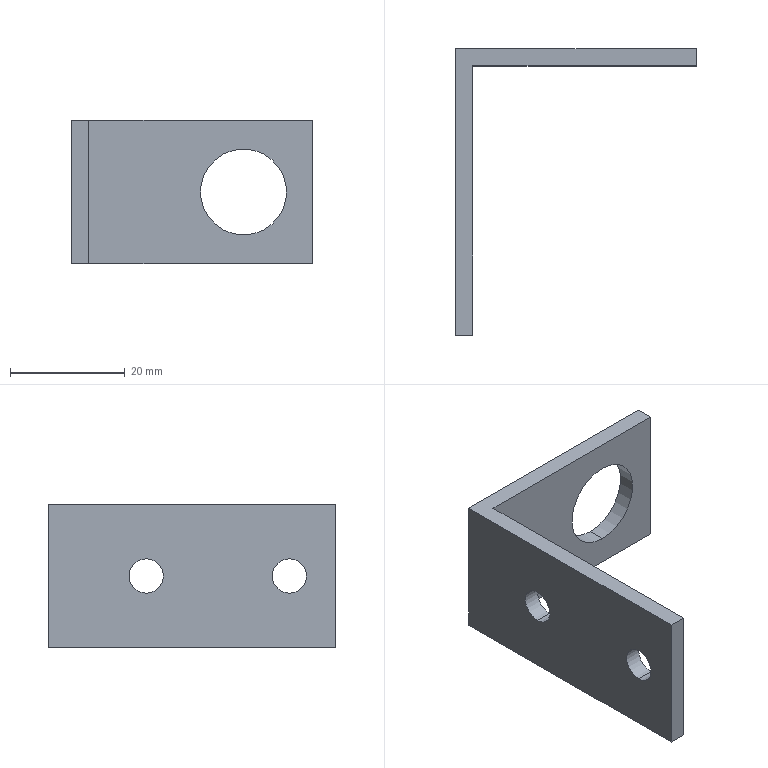Part | STEP file | 1 solid | 14 faces | box 42 x 50 x 25 mm | volume 5975 mm3 | plane 8 | cylinder 6 | commonest cylinder face diameters 6 x4 15 x2
STEP:
#1=CARTESIAN_POINT('',(0.,0.,0.));
#2=DIRECTION('',(0.,0.,1.));
#3=DIRECTION('',(1.,0.,0.));
#4=AXIS2_PLACEMENT_3D('',#1,#2,#3);
#5=CARTESIAN_POINT('',(0.,-17.,-3.));
#6=VERTEX_POINT('',#5);
#7=CARTESIAN_POINT('',(3.,-17.,-3.));
#8=VERTEX_POINT('',#7);
#9=CARTESIAN_POINT('',(25.,-17.,-3.));
#10=DIRECTION('',(1.,0.,0.));
#11=VECTOR('',#10,1.);
#12=LINE('',#9,#11);
#13=CARTESIAN_POINT('',(25.,-17.,0.));
#14=DIRECTION('',(1.,0.,0.));
#15=DIRECTION('',(0.,0.,-1.));
#16=AXIS2_PLACEMENT_3D('',#13,#14,#15);
#17=CYLINDRICAL_SURFACE('',#16,3.);
#18=CARTESIAN_POINT('',(6.283,0.));
#19=DIRECTION('',(0.,1.));
#20=VECTOR('',#19,1.);
#21=LINE('',#18,#20);
#22=(GEOMETRIC_REPRESENTATION_CONTEXT(2)PARAMETRIC_REPRESENTATION_CONTEXT()REPRESENTATION_CONTEXT('',''));
#23=DEFINITIONAL_REPRESENTATION('',(#21),#22);
#24=PCURVE('',#17,#23);
#25=CARTESIAN_POINT('',(25.,-17.,0.));
#26=DIRECTION('',(1.,0.,0.));
#27=DIRECTION('',(0.,0.,-1.));
#28=AXIS2_PLACEMENT_3D('',#25,#26,#27);
#29=CYLINDRICAL_SURFACE('',#28,3.);
#30=CARTESIAN_POINT('',(0.,0.));
#31=DIRECTION('',(0.,1.));
#32=VECTOR('',#31,1.);
#33=LINE('',#30,#32);
#34=(GEOMETRIC_REPRESENTATION_CONTEXT(2)PARAMETRIC_REPRESENTATION_CONTEXT()REPRESENTATION_CONTEXT('',''));
#35=DEFINITIONAL_REPRESENTATION('',(#33),#34);
#36=PCURVE('',#29,#35);
#37=SURFACE_CURVE('',#12,(#24,#36),.PCURVE_S1.);
#38=EDGE_CURVE('',#6,#8,#37,.T.);
#39=ORIENTED_EDGE('',*,*,#38,.T.);
#40=CARTESIAN_POINT('',(3.,-17.,3.));
#41=VERTEX_POINT('',#40);
#42=CARTESIAN_POINT('',(3.,-17.,0.));
#43=DIRECTION('',(-1.,0.,0.));
#44=DIRECTION('',(0.,0.,-1.));
#45=AXIS2_PLACEMENT_3D('',#42,#43,#44);
#46=CIRCLE('',#45,3.);
#47=CARTESIAN_POINT('',(6.283,-22.));
#48=DIRECTION('',(-1.,0.));
#49=VECTOR('',#48,1.);
#50=LINE('',#47,#49);
#51=(GEOMETRIC_REPRESENTATION_CONTEXT(2)PARAMETRIC_REPRESENTATION_CONTEXT()REPRESENTATION_CONTEXT('',''));
#52=DEFINITIONAL_REPRESENTATION('',(#50),#51);
#53=PCURVE('',#17,#52);
#54=CARTESIAN_POINT('',(3.,0.,-12.5));
#55=DIRECTION('',(-1.,0.,0.));
#56=DIRECTION('',(0.,-1.,0.));
#57=AXIS2_PLACEMENT_3D('',#54,#55,#56);
#58=PLANE('',#57);
#59=CARTESIAN_POINT('',(17.,12.5));
#60=DIRECTION('',(0.,-1.));
#61=AXIS2_PLACEMENT_2D('',#59,#60);
#62=CIRCLE('',#61,3.);
#63=(GEOMETRIC_REPRESENTATION_CONTEXT(2)PARAMETRIC_REPRESENTATION_CONTEXT()REPRESENTATION_CONTEXT('',''));
#64=DEFINITIONAL_REPRESENTATION('',(#62),#63);
#65=PCURVE('',#58,#64);
#66=SURFACE_CURVE('',#46,(#53,#65),.PCURVE_S1.);
#67=EDGE_CURVE('',#8,#41,#66,.T.);
#68=ORIENTED_EDGE('',*,*,#67,.T.);
#69=CARTESIAN_POINT('',(0.,-17.,3.));
#70=VERTEX_POINT('',#69);
#71=CARTESIAN_POINT('',(25.,-17.,3.));
#72=DIRECTION('',(1.,0.,0.));
#73=VECTOR('',#72,1.);
#74=LINE('',#71,#73);
#75=CARTESIAN_POINT('',(3.142,0.));
#76=DIRECTION('',(0.,1.));
#77=VECTOR('',#76,1.);
#78=LINE('',#75,#77);
#79=(GEOMETRIC_REPRESENTATION_CONTEXT(2)PARAMETRIC_REPRESENTATION_CONTEXT()REPRESENTATION_CONTEXT('',''));
#80=DEFINITIONAL_REPRESENTATION('',(#78),#79);
#81=PCURVE('',#17,#80);
#82=CARTESIAN_POINT('',(3.142,0.));
#83=DIRECTION('',(0.,1.));
#84=VECTOR('',#83,1.);
#85=LINE('',#82,#84);
#86=(GEOMETRIC_REPRESENTATION_CONTEXT(2)PARAMETRIC_REPRESENTATION_CONTEXT()REPRESENTATION_CONTEXT('',''));
#87=DEFINITIONAL_REPRESENTATION('',(#85),#86);
#88=PCURVE('',#29,#87);
#89=SURFACE_CURVE('',#74,(#81,#88),.PCURVE_S1.);
#90=EDGE_CURVE('',#70,#41,#89,.T.);
#91=ORIENTED_EDGE('',*,*,#90,.F.);
#92=CARTESIAN_POINT('',(0.,-17.,0.));
#93=DIRECTION('',(1.,0.,0.));
#94=DIRECTION('',(0.,0.,-1.));
#95=AXIS2_PLACEMENT_3D('',#92,#93,#94);
#96=CIRCLE('',#95,3.);
#97=CARTESIAN_POINT('',(0.,-25.));
#98=DIRECTION('',(1.,0.));
#99=VECTOR('',#98,1.);
#100=LINE('',#97,#99);
#101=(GEOMETRIC_REPRESENTATION_CONTEXT(2)PARAMETRIC_REPRESENTATION_CONTEXT()REPRESENTATION_CONTEXT('',''));
#102=DEFINITIONAL_REPRESENTATION('',(#100),#101);
#103=PCURVE('',#17,#102);
#104=CARTESIAN_POINT('',(0.,0.,-12.5));
#105=DIRECTION('',(-1.,0.,0.));
#106=DIRECTION('',(0.,-1.,0.));
#107=AXIS2_PLACEMENT_3D('',#104,#105,#106);
#108=PLANE('',#107);
#109=CARTESIAN_POINT('',(17.,9.5));
#110=CARTESIAN_POINT('',(11.804,9.5));
#111=CARTESIAN_POINT('',(14.402,14.));
#112=CARTESIAN_POINT('',(17.,18.5));
#113=CARTESIAN_POINT('',(19.598,14.));
#114=CARTESIAN_POINT('',(22.196,9.5));
#115=CARTESIAN_POINT('',(17.,9.5));
#116=(BOUNDED_CURVE()B_SPLINE_CURVE(2,(#109,#110,#111,#112,#113,#114,#115),.UNSPECIFIED.,.T.,.F.)B_SPLINE_CURVE_WITH_KNOTS((1,2,2,2,2,1),(-2.094,0.,2.094,4.189,6.283,8.378),.UNSPECIFIED.)CURVE()GEOMETRIC_REPRESENTATION_ITEM()RATIONAL_B_SPLINE_CURVE((1.,0.5,1.,0.5,1.,0.5,1.))REPRESENTATION_ITEM(''));
#117=(GEOMETRIC_REPRESENTATION_CONTEXT(2)PARAMETRIC_REPRESENTATION_CONTEXT()REPRESENTATION_CONTEXT('',''));
#118=DEFINITIONAL_REPRESENTATION('',(#116),#117);
#119=PCURVE('',#108,#118);
#120=SURFACE_CURVE('',#96,(#103,#119),.PCURVE_S1.);
#121=EDGE_CURVE('',#70,#6,#120,.T.);
#122=ORIENTED_EDGE('',*,*,#121,.T.);
#123=EDGE_LOOP('',(#39,#68,#91,#122));
#124=FACE_BOUND('',#123,.F.);
#125=ADVANCED_FACE('',(#124),#17,.F.);
#126=CARTESIAN_POINT('',(0.,-42.,-3.));
#127=VERTEX_POINT('',#126);
#128=CARTESIAN_POINT('',(3.,-42.,-3.));
#129=VERTEX_POINT('',#128);
#130=CARTESIAN_POINT('',(25.,-42.,-3.));
#131=DIRECTION('',(1.,0.,0.));
#132=VECTOR('',#131,1.);
#133=LINE('',#130,#132);
#134=CARTESIAN_POINT('',(25.,-42.,0.));
#135=DIRECTION('',(1.,0.,0.));
#136=DIRECTION('',(0.,0.,-1.));
#137=AXIS2_PLACEMENT_3D('',#134,#135,#136);
#138=CYLINDRICAL_SURFACE('',#137,3.);
#139=CARTESIAN_POINT('',(6.283,0.));
#140=DIRECTION('',(0.,1.));
#141=VECTOR('',#140,1.);
#142=LINE('',#139,#141);
#143=(GEOMETRIC_REPRESENTATION_CONTEXT(2)PARAMETRIC_REPRESENTATION_CONTEXT()REPRESENTATION_CONTEXT('',''));
#144=DEFINITIONAL_REPRESENTATION('',(#142),#143);
#145=PCURVE('',#138,#144);
#146=CARTESIAN_POINT('',(25.,-42.,0.));
#147=DIRECTION('',(1.,0.,0.));
#148=DIRECTION('',(0.,0.,-1.));
#149=AXIS2_PLACEMENT_3D('',#146,#147,#148);
#150=CYLINDRICAL_SURFACE('',#149,3.);
#151=CARTESIAN_POINT('',(0.,0.));
#152=DIRECTION('',(0.,1.));
#153=VECTOR('',#152,1.);
#154=LINE('',#151,#153);
#155=(GEOMETRIC_REPRESENTATION_CONTEXT(2)PARAMETRIC_REPRESENTATION_CONTEXT()REPRESENTATION_CONTEXT('',''));
#156=DEFINITIONAL_REPRESENTATION('',(#154),#155);
#157=PCURVE('',#150,#156);
#158=SURFACE_CURVE('',#133,(#145,#157),.PCURVE_S1.);
#159=EDGE_CURVE('',#127,#129,#158,.T.);
#160=ORIENTED_EDGE('',*,*,#159,.T.);
#161=CARTESIAN_POINT('',(3.,-42.,3.));
#162=VERTEX_POINT('',#161);
#163=CARTESIAN_POINT('',(3.,-42.,0.));
#164=DIRECTION('',(-1.,0.,0.));
#165=DIRECTION('',(0.,0.,-1.));
#166=AXIS2_PLACEMENT_3D('',#163,#164,#165);
#167=CIRCLE('',#166,3.);
#168=CARTESIAN_POINT('',(6.283,-22.));
#169=DIRECTION('',(-1.,0.));
#170=VECTOR('',#169,1.);
#171=LINE('',#168,#170);
#172=(GEOMETRIC_REPRESENTATION_CONTEXT(2)PARAMETRIC_REPRESENTATION_CONTEXT()REPRESENTATION_CONTEXT('',''));
#173=DEFINITIONAL_REPRESENTATION('',(#171),#172);
#174=PCURVE('',#138,#173);
#175=CARTESIAN_POINT('',(42.,12.5));
#176=DIRECTION('',(0.,-1.));
#177=AXIS2_PLACEMENT_2D('',#175,#176);
#178=CIRCLE('',#177,3.);
#179=(GEOMETRIC_REPRESENTATION_CONTEXT(2)PARAMETRIC_REPRESENTATION_CONTEXT()REPRESENTATION_CONTEXT('',''));
#180=DEFINITIONAL_REPRESENTATION('',(#178),#179);
#181=PCURVE('',#58,#180);
#182=SURFACE_CURVE('',#167,(#174,#181),.PCURVE_S1.);
#183=EDGE_CURVE('',#129,#162,#182,.T.);
#184=ORIENTED_EDGE('',*,*,#183,.T.);
#185=CARTESIAN_POINT('',(0.,-42.,3.));
#186=VERTEX_POINT('',#185);
#187=CARTESIAN_POINT('',(25.,-42.,3.));
#188=DIRECTION('',(1.,0.,0.));
#189=VECTOR('',#188,1.);
#190=LINE('',#187,#189);
#191=CARTESIAN_POINT('',(3.142,0.));
#192=DIRECTION('',(0.,1.));
#193=VECTOR('',#192,1.);
#194=LINE('',#191,#193);
#195=(GEOMETRIC_REPRESENTATION_CONTEXT(2)PARAMETRIC_REPRESENTATION_CONTEXT()REPRESENTATION_CONTEXT('',''));
#196=DEFINITIONAL_REPRESENTATION('',(#194),#195);
#197=PCURVE('',#138,#196);
#198=CARTESIAN_POINT('',(3.142,0.));
#199=DIRECTION('',(0.,1.));
#200=VECTOR('',#199,1.);
#201=LINE('',#198,#200);
#202=(GEOMETRIC_REPRESENTATION_CONTEXT(2)PARAMETRIC_REPRESENTATION_CONTEXT()REPRESENTATION_CONTEXT('',''));
#203=DEFINITIONAL_REPRESENTATION('',(#201),#202);
#204=PCURVE('',#150,#203);
#205=SURFACE_CURVE('',#190,(#197,#204),.PCURVE_S1.);
#206=EDGE_CURVE('',#186,#162,#205,.T.);
#207=ORIENTED_EDGE('',*,*,#206,.F.);
#208=CARTESIAN_POINT('',(0.,-42.,0.));
#209=DIRECTION('',(1.,0.,0.));
#210=DIRECTION('',(0.,0.,-1.));
#211=AXIS2_PLACEMENT_3D('',#208,#209,#210);
#212=CIRCLE('',#211,3.);
#213=CARTESIAN_POINT('',(0.,-25.));
#214=DIRECTION('',(1.,0.));
#215=VECTOR('',#214,1.);
#216=LINE('',#213,#215);
#217=(GEOMETRIC_REPRESENTATION_CONTEXT(2)PARAMETRIC_REPRESENTATION_CONTEXT()REPRESENTATION_CONTEXT('',''));
#218=DEFINITIONAL_REPRESENTATION('',(#216),#217);
#219=PCURVE('',#138,#218);
#220=CARTESIAN_POINT('',(42.,9.5));
#221=CARTESIAN_POINT('',(36.804,9.5));
#222=CARTESIAN_POINT('',(39.402,14.));
#223=CARTESIAN_POINT('',(42.,18.5));
#224=CARTESIAN_POINT('',(44.598,14.));
#225=CARTESIAN_POINT('',(47.196,9.5));
#226=CARTESIAN_POINT('',(42.,9.5));
#227=(BOUNDED_CURVE()B_SPLINE_CURVE(2,(#220,#221,#222,#223,#224,#225,#226),.UNSPECIFIED.,.T.,.F.)B_SPLINE_CURVE_WITH_KNOTS((1,2,2,2,2,1),(-2.094,0.,2.094,4.189,6.283,8.378),.UNSPECIFIED.)CURVE()GEOMETRIC_REPRESENTATION_ITEM()RATIONAL_B_SPLINE_CURVE((1.,0.5,1.,0.5,1.,0.5,1.))REPRESENTATION_ITEM(''));
#228=(GEOMETRIC_REPRESENTATION_CONTEXT(2)PARAMETRIC_REPRESENTATION_CONTEXT()REPRESENTATION_CONTEXT('',''));
#229=DEFINITIONAL_REPRESENTATION('',(#227),#228);
#230=PCURVE('',#108,#229);
#231=SURFACE_CURVE('',#212,(#219,#230),.PCURVE_S1.);
#232=EDGE_CURVE('',#186,#127,#231,.T.);
#233=ORIENTED_EDGE('',*,*,#232,.T.);
#234=EDGE_LOOP('',(#160,#184,#207,#233));
#235=FACE_BOUND('',#234,.F.);
#236=ADVANCED_FACE('',(#235),#138,.F.);
#237=CARTESIAN_POINT('',(30.,0.,-7.5));
#238=VERTEX_POINT('',#237);
#239=CARTESIAN_POINT('',(30.,-3.,-7.5));
#240=VERTEX_POINT('',#239);
#241=CARTESIAN_POINT('',(30.,-25.,-7.5));
#242=DIRECTION('',(0.,-1.,0.));
#243=VECTOR('',#242,1.);
#244=LINE('',#241,#243);
#245=CARTESIAN_POINT('',(30.,-25.,0.));
#246=DIRECTION('',(0.,-1.,0.));
#247=DIRECTION('',(0.,0.,-1.));
#248=AXIS2_PLACEMENT_3D('',#245,#246,#247);
#249=CYLINDRICAL_SURFACE('',#248,7.5);
#250=CARTESIAN_POINT('',(6.283,0.));
#251=DIRECTION('',(0.,1.));
#252=VECTOR('',#251,1.);
#253=LINE('',#250,#252);
#254=(GEOMETRIC_REPRESENTATION_CONTEXT(2)PARAMETRIC_REPRESENTATION_CONTEXT()REPRESENTATION_CONTEXT('',''));
#255=DEFINITIONAL_REPRESENTATION('',(#253),#254);
#256=PCURVE('',#249,#255);
#257=CARTESIAN_POINT('',(30.,-25.,0.));
#258=DIRECTION('',(0.,-1.,0.));
#259=DIRECTION('',(0.,0.,-1.));
#260=AXIS2_PLACEMENT_3D('',#257,#258,#259);
#261=CYLINDRICAL_SURFACE('',#260,7.5);
#262=CARTESIAN_POINT('',(0.,0.));
#263=DIRECTION('',(0.,1.));
#264=VECTOR('',#263,1.);
#265=LINE('',#262,#264);
#266=(GEOMETRIC_REPRESENTATION_CONTEXT(2)PARAMETRIC_REPRESENTATION_CONTEXT()REPRESENTATION_CONTEXT('',''));
#267=DEFINITIONAL_REPRESENTATION('',(#265),#266);
#268=PCURVE('',#261,#267);
#269=SURFACE_CURVE('',#244,(#256,#268),.PCURVE_S1.);
#270=EDGE_CURVE('',#238,#240,#269,.T.);
#271=ORIENTED_EDGE('',*,*,#270,.T.);
#272=CARTESIAN_POINT('',(30.,-3.,7.5));
#273=VERTEX_POINT('',#272);
#274=CARTESIAN_POINT('',(30.,-3.,0.));
#275=DIRECTION('',(0.,1.,0.));
#276=DIRECTION('',(0.,0.,-1.));
#277=AXIS2_PLACEMENT_3D('',#274,#275,#276);
#278=CIRCLE('',#277,7.5);
#279=CARTESIAN_POINT('',(6.283,-22.));
#280=DIRECTION('',(-1.,0.));
#281=VECTOR('',#280,1.);
#282=LINE('',#279,#281);
#283=(GEOMETRIC_REPRESENTATION_CONTEXT(2)PARAMETRIC_REPRESENTATION_CONTEXT()REPRESENTATION_CONTEXT('',''));
#284=DEFINITIONAL_REPRESENTATION('',(#282),#283);
#285=PCURVE('',#249,#284);
#286=CARTESIAN_POINT('',(0.,-3.,-12.5));
#287=DIRECTION('',(0.,1.,0.));
#288=DIRECTION('',(0.,0.,1.));
#289=AXIS2_PLACEMENT_3D('',#286,#287,#288);
#290=PLANE('',#289);
#291=CARTESIAN_POINT('',(12.5,30.));
#292=DIRECTION('',(-1.,0.));
#293=AXIS2_PLACEMENT_2D('',#291,#292);
#294=CIRCLE('',#293,7.5);
#295=(GEOMETRIC_REPRESENTATION_CONTEXT(2)PARAMETRIC_REPRESENTATION_CONTEXT()REPRESENTATION_CONTEXT('',''));
#296=DEFINITIONAL_REPRESENTATION('',(#294),#295);
#297=PCURVE('',#290,#296);
#298=SURFACE_CURVE('',#278,(#285,#297),.PCURVE_S1.);
#299=EDGE_CURVE('',#240,#273,#298,.T.);
#300=ORIENTED_EDGE('',*,*,#299,.T.);
#301=CARTESIAN_POINT('',(30.,0.,7.5));
#302=VERTEX_POINT('',#301);
#303=CARTESIAN_POINT('',(30.,-25.,7.5));
#304=DIRECTION('',(0.,-1.,0.));
#305=VECTOR('',#304,1.);
#306=LINE('',#303,#305);
#307=CARTESIAN_POINT('',(3.142,0.));
#308=DIRECTION('',(0.,1.));
#309=VECTOR('',#308,1.);
#310=LINE('',#307,#309);
#311=(GEOMETRIC_REPRESENTATION_CONTEXT(2)PARAMETRIC_REPRESENTATION_CONTEXT()REPRESENTATION_CONTEXT('',''));
#312=DEFINITIONAL_REPRESENTATION('',(#310),#311);
#313=PCURVE('',#249,#312);
#314=CARTESIAN_POINT('',(3.142,0.));
#315=DIRECTION('',(0.,1.));
#316=VECTOR('',#315,1.);
#317=LINE('',#314,#316);
#318=(GEOMETRIC_REPRESENTATION_CONTEXT(2)PARAMETRIC_REPRESENTATION_CONTEXT()REPRESENTATION_CONTEXT('',''));
#319=DEFINITIONAL_REPRESENTATION('',(#317),#318);
#320=PCURVE('',#261,#319);
#321=SURFACE_CURVE('',#306,(#313,#320),.PCURVE_S1.);
#322=EDGE_CURVE('',#302,#273,#321,.T.);
#323=ORIENTED_EDGE('',*,*,#322,.F.);
#324=CARTESIAN_POINT('',(30.,0.,0.));
#325=DIRECTION('',(0.,-1.,0.));
#326=DIRECTION('',(0.,0.,-1.));
#327=AXIS2_PLACEMENT_3D('',#324,#325,#326);
#328=CIRCLE('',#327,7.5);
#329=CARTESIAN_POINT('',(0.,-25.));
#330=DIRECTION('',(1.,0.));
#331=VECTOR('',#330,1.);
#332=LINE('',#329,#331);
#333=(GEOMETRIC_REPRESENTATION_CONTEXT(2)PARAMETRIC_REPRESENTATION_CONTEXT()REPRESENTATION_CONTEXT('',''));
#334=DEFINITIONAL_REPRESENTATION('',(#332),#333);
#335=PCURVE('',#249,#334);
#336=CARTESIAN_POINT('',(0.,0.,-12.5));
#337=DIRECTION('',(0.,1.,0.));
#338=DIRECTION('',(0.,0.,1.));
#339=AXIS2_PLACEMENT_3D('',#336,#337,#338);
#340=PLANE('',#339);
#341=CARTESIAN_POINT('',(5.,30.));
#342=CARTESIAN_POINT('',(5.,42.99));
#343=CARTESIAN_POINT('',(16.25,36.495));
#344=CARTESIAN_POINT('',(27.5,30.));
#345=CARTESIAN_POINT('',(16.25,23.505));
#346=CARTESIAN_POINT('',(5.,17.01));
#347=CARTESIAN_POINT('',(5.,30.));
#348=(BOUNDED_CURVE()B_SPLINE_CURVE(2,(#341,#342,#343,#344,#345,#346,#347),.UNSPECIFIED.,.T.,.F.)B_SPLINE_CURVE_WITH_KNOTS((1,2,2,2,2,1),(-2.094,0.,2.094,4.189,6.283,8.378),.UNSPECIFIED.)CURVE()GEOMETRIC_REPRESENTATION_ITEM()RATIONAL_B_SPLINE_CURVE((1.,0.5,1.,0.5,1.,0.5,1.))REPRESENTATION_ITEM(''));
#349=(GEOMETRIC_REPRESENTATION_CONTEXT(2)PARAMETRIC_REPRESENTATION_CONTEXT()REPRESENTATION_CONTEXT('',''));
#350=DEFINITIONAL_REPRESENTATION('',(#348),#349);
#351=PCURVE('',#340,#350);
#352=SURFACE_CURVE('',#328,(#335,#351),.PCURVE_S1.);
#353=EDGE_CURVE('',#302,#238,#352,.T.);
#354=ORIENTED_EDGE('',*,*,#353,.T.);
#355=EDGE_LOOP('',(#271,#300,#323,#354));
#356=FACE_BOUND('',#355,.F.);
#357=ADVANCED_FACE('',(#356),#249,.F.);
#358=CARTESIAN_POINT('',(0.,-17.,0.));
#359=DIRECTION('',(1.,0.,0.));
#360=DIRECTION('',(0.,0.,-1.));
#361=AXIS2_PLACEMENT_3D('',#358,#359,#360);
#362=CIRCLE('',#361,3.);
#363=CARTESIAN_POINT('',(17.,9.5));
#364=CARTESIAN_POINT('',(11.804,9.5));
#365=CARTESIAN_POINT('',(14.402,14.));
#366=CARTESIAN_POINT('',(17.,18.5));
#367=CARTESIAN_POINT('',(19.598,14.));
#368=CARTESIAN_POINT('',(22.196,9.5));
#369=CARTESIAN_POINT('',(17.,9.5));
#370=(BOUNDED_CURVE()B_SPLINE_CURVE(2,(#363,#364,#365,#366,#367,#368,#369),.UNSPECIFIED.,.T.,.F.)B_SPLINE_CURVE_WITH_KNOTS((1,2,2,2,2,1),(-2.094,0.,2.094,4.189,6.283,8.378),.UNSPECIFIED.)CURVE()GEOMETRIC_REPRESENTATION_ITEM()RATIONAL_B_SPLINE_CURVE((1.,0.5,1.,0.5,1.,0.5,1.))REPRESENTATION_ITEM(''));
#371=(GEOMETRIC_REPRESENTATION_CONTEXT(2)PARAMETRIC_REPRESENTATION_CONTEXT()REPRESENTATION_CONTEXT('',''));
#372=DEFINITIONAL_REPRESENTATION('',(#370),#371);
#373=PCURVE('',#108,#372);
#374=CARTESIAN_POINT('',(0.,-25.));
#375=DIRECTION('',(1.,0.));
#376=VECTOR('',#375,1.);
#377=LINE('',#374,#376);
#378=(GEOMETRIC_REPRESENTATION_CONTEXT(2)PARAMETRIC_REPRESENTATION_CONTEXT()REPRESENTATION_CONTEXT('',''));
#379=DEFINITIONAL_REPRESENTATION('',(#377),#378);
#380=PCURVE('',#29,#379);
#381=SURFACE_CURVE('',#362,(#373,#380),.PCURVE_S1.);
#382=EDGE_CURVE('',#6,#70,#381,.T.);
#383=ORIENTED_EDGE('',*,*,#382,.T.);
#384=ORIENTED_EDGE('',*,*,#121,.T.);
#385=EDGE_LOOP('',(#383,#384));
#386=FACE_BOUND('',#385,.T.);
#387=CARTESIAN_POINT('',(0.,-42.,0.));
#388=DIRECTION('',(1.,0.,0.));
#389=DIRECTION('',(0.,0.,-1.));
#390=AXIS2_PLACEMENT_3D('',#387,#388,#389);
#391=CIRCLE('',#390,3.);
#392=CARTESIAN_POINT('',(42.,9.5));
#393=CARTESIAN_POINT('',(36.804,9.5));
#394=CARTESIAN_POINT('',(39.402,14.));
#395=CARTESIAN_POINT('',(42.,18.5));
#396=CARTESIAN_POINT('',(44.598,14.));
#397=CARTESIAN_POINT('',(47.196,9.5));
#398=CARTESIAN_POINT('',(42.,9.5));
#399=(BOUNDED_CURVE()B_SPLINE_CURVE(2,(#392,#393,#394,#395,#396,#397,#398),.UNSPECIFIED.,.T.,.F.)B_SPLINE_CURVE_WITH_KNOTS((1,2,2,2,2,1),(-2.094,0.,2.094,4.189,6.283,8.378),.UNSPECIFIED.)CURVE()GEOMETRIC_REPRESENTATION_ITEM()RATIONAL_B_SPLINE_CURVE((1.,0.5,1.,0.5,1.,0.5,1.))REPRESENTATION_ITEM(''));
#400=(GEOMETRIC_REPRESENTATION_CONTEXT(2)PARAMETRIC_REPRESENTATION_CONTEXT()REPRESENTATION_CONTEXT('',''));
#401=DEFINITIONAL_REPRESENTATION('',(#399),#400);
#402=PCURVE('',#108,#401);
#403=CARTESIAN_POINT('',(0.,-25.));
#404=DIRECTION('',(1.,0.));
#405=VECTOR('',#404,1.);
#406=LINE('',#403,#405);
#407=(GEOMETRIC_REPRESENTATION_CONTEXT(2)PARAMETRIC_REPRESENTATION_CONTEXT()REPRESENTATION_CONTEXT('',''));
#408=DEFINITIONAL_REPRESENTATION('',(#406),#407);
#409=PCURVE('',#150,#408);
#410=SURFACE_CURVE('',#391,(#402,#409),.PCURVE_S1.);
#411=EDGE_CURVE('',#127,#186,#410,.T.);
#412=ORIENTED_EDGE('',*,*,#411,.T.);
#413=ORIENTED_EDGE('',*,*,#232,.T.);
#414=EDGE_LOOP('',(#412,#413));
#415=FACE_BOUND('',#414,.T.);
#416=CARTESIAN_POINT('',(0.,-50.,12.5));
#417=VERTEX_POINT('',#416);
#418=CARTESIAN_POINT('',(0.,0.,12.5));
#419=VERTEX_POINT('',#418);
#420=CARTESIAN_POINT('',(0.,0.,12.5));
#421=DIRECTION('',(0.,1.,0.));
#422=VECTOR('',#421,1.);
#423=LINE('',#420,#422);
#424=CARTESIAN_POINT('',(0.,25.));
#425=DIRECTION('',(-1.,0.));
#426=VECTOR('',#425,1.);
#427=LINE('',#424,#426);
#428=(GEOMETRIC_REPRESENTATION_CONTEXT(2)PARAMETRIC_REPRESENTATION_CONTEXT()REPRESENTATION_CONTEXT('',''));
#429=DEFINITIONAL_REPRESENTATION('',(#427),#428);
#430=PCURVE('',#108,#429);
#431=CARTESIAN_POINT('',(0.,-50.,12.5));
#432=DIRECTION('',(0.,0.,-1.));
#433=DIRECTION('',(-1.,0.,0.));
#434=AXIS2_PLACEMENT_3D('',#431,#432,#433);
#435=PLANE('',#434);
#436=CARTESIAN_POINT('',(0.,50.));
#437=DIRECTION('',(0.,1.));
#438=VECTOR('',#437,1.);
#439=LINE('',#436,#438);
#440=(GEOMETRIC_REPRESENTATION_CONTEXT(2)PARAMETRIC_REPRESENTATION_CONTEXT()REPRESENTATION_CONTEXT('',''));
#441=DEFINITIONAL_REPRESENTATION('',(#439),#440);
#442=PCURVE('',#435,#441);
#443=SURFACE_CURVE('',#423,(#430,#442),.PCURVE_S1.);
#444=EDGE_CURVE('',#417,#419,#443,.T.);
#445=ORIENTED_EDGE('',*,*,#444,.T.);
#446=CARTESIAN_POINT('',(0.,0.,-12.5));
#447=VERTEX_POINT('',#446);
#448=CARTESIAN_POINT('',(0.,0.,-12.5));
#449=DIRECTION('',(0.,0.,-1.));
#450=VECTOR('',#449,1.);
#451=LINE('',#448,#450);
#452=CARTESIAN_POINT('',(0.,0.));
#453=DIRECTION('',(0.,-1.));
#454=VECTOR('',#453,1.);
#455=LINE('',#452,#454);
#456=(GEOMETRIC_REPRESENTATION_CONTEXT(2)PARAMETRIC_REPRESENTATION_CONTEXT()REPRESENTATION_CONTEXT('',''));
#457=DEFINITIONAL_REPRESENTATION('',(#455),#456);
#458=PCURVE('',#108,#457);
#459=CARTESIAN_POINT('',(0.,0.));
#460=DIRECTION('',(-1.,0.));
#461=VECTOR('',#460,1.);
#462=LINE('',#459,#461);
#463=(GEOMETRIC_REPRESENTATION_CONTEXT(2)PARAMETRIC_REPRESENTATION_CONTEXT()REPRESENTATION_CONTEXT('',''));
#464=DEFINITIONAL_REPRESENTATION('',(#462),#463);
#465=PCURVE('',#340,#464);
#466=SURFACE_CURVE('',#451,(#458,#465),.PCURVE_S1.);
#467=EDGE_CURVE('',#419,#447,#466,.T.);
#468=ORIENTED_EDGE('',*,*,#467,.T.);
#469=CARTESIAN_POINT('',(0.,-50.,-12.5));
#470=VERTEX_POINT('',#469);
#471=CARTESIAN_POINT('',(0.,0.,-12.5));
#472=DIRECTION('',(0.,-1.,0.));
#473=VECTOR('',#472,1.);
#474=LINE('',#471,#473);
#475=CARTESIAN_POINT('',(0.,0.));
#476=DIRECTION('',(1.,0.));
#477=VECTOR('',#476,1.);
#478=LINE('',#475,#477);
#479=(GEOMETRIC_REPRESENTATION_CONTEXT(2)PARAMETRIC_REPRESENTATION_CONTEXT()REPRESENTATION_CONTEXT('',''));
#480=DEFINITIONAL_REPRESENTATION('',(#478),#479);
#481=PCURVE('',#108,#480);
#482=CARTESIAN_POINT('',(0.,-50.,-12.5));
#483=DIRECTION('',(0.,0.,-1.));
#484=DIRECTION('',(-1.,0.,0.));
#485=AXIS2_PLACEMENT_3D('',#482,#483,#484);
#486=PLANE('',#485);
#487=CARTESIAN_POINT('',(0.,50.));
#488=DIRECTION('',(0.,-1.));
#489=VECTOR('',#488,1.);
#490=LINE('',#487,#489);
#491=(GEOMETRIC_REPRESENTATION_CONTEXT(2)PARAMETRIC_REPRESENTATION_CONTEXT()REPRESENTATION_CONTEXT('',''));
#492=DEFINITIONAL_REPRESENTATION('',(#490),#491);
#493=PCURVE('',#486,#492);
#494=SURFACE_CURVE('',#474,(#481,#493),.PCURVE_S1.);
#495=EDGE_CURVE('',#447,#470,#494,.T.);
#496=ORIENTED_EDGE('',*,*,#495,.T.);
#497=CARTESIAN_POINT('',(0.,-50.,-12.5));
#498=DIRECTION('',(0.,0.,1.));
#499=VECTOR('',#498,1.);
#500=LINE('',#497,#499);
#501=CARTESIAN_POINT('',(50.,0.));
#502=DIRECTION('',(0.,1.));
#503=VECTOR('',#502,1.);
#504=LINE('',#501,#503);
#505=(GEOMETRIC_REPRESENTATION_CONTEXT(2)PARAMETRIC_REPRESENTATION_CONTEXT()REPRESENTATION_CONTEXT('',''));
#506=DEFINITIONAL_REPRESENTATION('',(#504),#505);
#507=PCURVE('',#108,#506);
#508=CARTESIAN_POINT('',(3.,-50.,-12.5));
#509=DIRECTION('',(0.,1.,0.));
#510=DIRECTION('',(0.,0.,1.));
#511=AXIS2_PLACEMENT_3D('',#508,#509,#510);
#512=PLANE('',#511);
#513=CARTESIAN_POINT('',(0.,-3.));
#514=DIRECTION('',(1.,0.));
#515=VECTOR('',#514,1.);
#516=LINE('',#513,#515);
#517=(GEOMETRIC_REPRESENTATION_CONTEXT(2)PARAMETRIC_REPRESENTATION_CONTEXT()REPRESENTATION_CONTEXT('',''));
#518=DEFINITIONAL_REPRESENTATION('',(#516),#517);
#519=PCURVE('',#512,#518);
#520=SURFACE_CURVE('',#500,(#507,#519),.PCURVE_S1.);
#521=EDGE_CURVE('',#470,#417,#520,.T.);
#522=ORIENTED_EDGE('',*,*,#521,.T.);
#523=EDGE_LOOP('',(#445,#468,#496,#522));
#524=FACE_BOUND('',#523,.T.);
#525=ADVANCED_FACE('',(#386,#415,#524),#108,.T.);
#526=CARTESIAN_POINT('',(3.,-17.,0.));
#527=DIRECTION('',(-1.,0.,0.));
#528=DIRECTION('',(0.,0.,-1.));
#529=AXIS2_PLACEMENT_3D('',#526,#527,#528);
#530=CIRCLE('',#529,3.);
#531=CARTESIAN_POINT('',(6.283,-22.));
#532=DIRECTION('',(-1.,0.));
#533=VECTOR('',#532,1.);
#534=LINE('',#531,#533);
#535=(GEOMETRIC_REPRESENTATION_CONTEXT(2)PARAMETRIC_REPRESENTATION_CONTEXT()REPRESENTATION_CONTEXT('',''));
#536=DEFINITIONAL_REPRESENTATION('',(#534),#535);
#537=PCURVE('',#29,#536);
#538=CARTESIAN_POINT('',(17.,12.5));
#539=DIRECTION('',(0.,-1.));
#540=AXIS2_PLACEMENT_2D('',#538,#539);
#541=CIRCLE('',#540,3.);
#542=(GEOMETRIC_REPRESENTATION_CONTEXT(2)PARAMETRIC_REPRESENTATION_CONTEXT()REPRESENTATION_CONTEXT('',''));
#543=DEFINITIONAL_REPRESENTATION('',(#541),#542);
#544=PCURVE('',#58,#543);
#545=SURFACE_CURVE('',#530,(#537,#544),.PCURVE_S1.);
#546=EDGE_CURVE('',#41,#8,#545,.T.);
#547=ORIENTED_EDGE('',*,*,#546,.T.);
#548=ORIENTED_EDGE('',*,*,#38,.F.);
#549=ORIENTED_EDGE('',*,*,#382,.T.);
#550=ORIENTED_EDGE('',*,*,#90,.T.);
#551=EDGE_LOOP('',(#547,#548,#549,#550));
#552=FACE_BOUND('',#551,.F.);
#553=ADVANCED_FACE('',(#552),#29,.F.);
#554=CARTESIAN_POINT('',(3.,-42.,0.));
#555=DIRECTION('',(-1.,0.,0.));
#556=DIRECTION('',(0.,0.,-1.));
#557=AXIS2_PLACEMENT_3D('',#554,#555,#556);
#558=CIRCLE('',#557,3.);
#559=CARTESIAN_POINT('',(6.283,-22.));
#560=DIRECTION('',(-1.,0.));
#561=VECTOR('',#560,1.);
#562=LINE('',#559,#561);
#563=(GEOMETRIC_REPRESENTATION_CONTEXT(2)PARAMETRIC_REPRESENTATION_CONTEXT()REPRESENTATION_CONTEXT('',''));
#564=DEFINITIONAL_REPRESENTATION('',(#562),#563);
#565=PCURVE('',#150,#564);
#566=CARTESIAN_POINT('',(42.,12.5));
#567=DIRECTION('',(0.,-1.));
#568=AXIS2_PLACEMENT_2D('',#566,#567);
#569=CIRCLE('',#568,3.);
#570=(GEOMETRIC_REPRESENTATION_CONTEXT(2)PARAMETRIC_REPRESENTATION_CONTEXT()REPRESENTATION_CONTEXT('',''));
#571=DEFINITIONAL_REPRESENTATION('',(#569),#570);
#572=PCURVE('',#58,#571);
#573=SURFACE_CURVE('',#558,(#565,#572),.PCURVE_S1.);
#574=EDGE_CURVE('',#162,#129,#573,.T.);
#575=ORIENTED_EDGE('',*,*,#574,.T.);
#576=ORIENTED_EDGE('',*,*,#159,.F.);
#577=ORIENTED_EDGE('',*,*,#411,.T.);
#578=ORIENTED_EDGE('',*,*,#206,.T.);
#579=EDGE_LOOP('',(#575,#576,#577,#578));
#580=FACE_BOUND('',#579,.F.);
#581=ADVANCED_FACE('',(#580),#150,.F.);
#582=CARTESIAN_POINT('',(30.,0.,0.));
#583=DIRECTION('',(0.,-1.,0.));
#584=DIRECTION('',(0.,0.,-1.));
#585=AXIS2_PLACEMENT_3D('',#582,#583,#584);
#586=CIRCLE('',#585,7.5);
#587=CARTESIAN_POINT('',(5.,30.));
#588=CARTESIAN_POINT('',(5.,42.99));
#589=CARTESIAN_POINT('',(16.25,36.495));
#590=CARTESIAN_POINT('',(27.5,30.));
#591=CARTESIAN_POINT('',(16.25,23.505));
#592=CARTESIAN_POINT('',(5.,17.01));
#593=CARTESIAN_POINT('',(5.,30.));
#594=(BOUNDED_CURVE()B_SPLINE_CURVE(2,(#587,#588,#589,#590,#591,#592,#593),.UNSPECIFIED.,.T.,.F.)B_SPLINE_CURVE_WITH_KNOTS((1,2,2,2,2,1),(-2.094,0.,2.094,4.189,6.283,8.378),.UNSPECIFIED.)CURVE()GEOMETRIC_REPRESENTATION_ITEM()RATIONAL_B_SPLINE_CURVE((1.,0.5,1.,0.5,1.,0.5,1.))REPRESENTATION_ITEM(''));
#595=(GEOMETRIC_REPRESENTATION_CONTEXT(2)PARAMETRIC_REPRESENTATION_CONTEXT()REPRESENTATION_CONTEXT('',''));
#596=DEFINITIONAL_REPRESENTATION('',(#594),#595);
#597=PCURVE('',#340,#596);
#598=CARTESIAN_POINT('',(0.,-25.));
#599=DIRECTION('',(1.,0.));
#600=VECTOR('',#599,1.);
#601=LINE('',#598,#600);
#602=(GEOMETRIC_REPRESENTATION_CONTEXT(2)PARAMETRIC_REPRESENTATION_CONTEXT()REPRESENTATION_CONTEXT('',''));
#603=DEFINITIONAL_REPRESENTATION('',(#601),#602);
#604=PCURVE('',#261,#603);
#605=SURFACE_CURVE('',#586,(#597,#604),.PCURVE_S1.);
#606=EDGE_CURVE('',#238,#302,#605,.T.);
#607=ORIENTED_EDGE('',*,*,#606,.T.);
#608=ORIENTED_EDGE('',*,*,#353,.T.);
#609=EDGE_LOOP('',(#607,#608));
#610=FACE_BOUND('',#609,.T.);
#611=CARTESIAN_POINT('',(42.,0.,12.5));
#612=VERTEX_POINT('',#611);
#613=CARTESIAN_POINT('',(0.,0.,12.5));
#614=DIRECTION('',(1.,0.,0.));
#615=VECTOR('',#614,1.);
#616=LINE('',#613,#615);
#617=CARTESIAN_POINT('',(25.,0.));
#618=DIRECTION('',(0.,1.));
#619=VECTOR('',#618,1.);
#620=LINE('',#617,#619);
#621=(GEOMETRIC_REPRESENTATION_CONTEXT(2)PARAMETRIC_REPRESENTATION_CONTEXT()REPRESENTATION_CONTEXT('',''));
#622=DEFINITIONAL_REPRESENTATION('',(#620),#621);
#623=PCURVE('',#340,#622);
#624=CARTESIAN_POINT('',(0.,50.));
#625=DIRECTION('',(-1.,0.));
#626=VECTOR('',#625,1.);
#627=LINE('',#624,#626);
#628=(GEOMETRIC_REPRESENTATION_CONTEXT(2)PARAMETRIC_REPRESENTATION_CONTEXT()REPRESENTATION_CONTEXT('',''));
#629=DEFINITIONAL_REPRESENTATION('',(#627),#628);
#630=PCURVE('',#435,#629);
#631=SURFACE_CURVE('',#616,(#623,#630),.PCURVE_S1.);
#632=EDGE_CURVE('',#419,#612,#631,.T.);
#633=ORIENTED_EDGE('',*,*,#632,.T.);
#634=CARTESIAN_POINT('',(42.,0.,-12.5));
#635=VERTEX_POINT('',#634);
#636=CARTESIAN_POINT('',(42.,0.,-12.5));
#637=DIRECTION('',(0.,0.,-1.));
#638=VECTOR('',#637,1.);
#639=LINE('',#636,#638);
#640=CARTESIAN_POINT('',(0.,42.));
#641=DIRECTION('',(-1.,0.));
#642=VECTOR('',#641,1.);
#643=LINE('',#640,#642);
#644=(GEOMETRIC_REPRESENTATION_CONTEXT(2)PARAMETRIC_REPRESENTATION_CONTEXT()REPRESENTATION_CONTEXT('',''));
#645=DEFINITIONAL_REPRESENTATION('',(#643),#644);
#646=PCURVE('',#340,#645);
#647=CARTESIAN_POINT('',(42.,0.,-12.5));
#648=DIRECTION('',(-1.,0.,0.));
#649=DIRECTION('',(0.,0.,1.));
#650=AXIS2_PLACEMENT_3D('',#647,#648,#649);
#651=PLANE('',#650);
#652=CARTESIAN_POINT('',(0.,0.));
#653=DIRECTION('',(-1.,0.));
#654=VECTOR('',#653,1.);
#655=LINE('',#652,#654);
#656=(GEOMETRIC_REPRESENTATION_CONTEXT(2)PARAMETRIC_REPRESENTATION_CONTEXT()REPRESENTATION_CONTEXT('',''));
#657=DEFINITIONAL_REPRESENTATION('',(#655),#656);
#658=PCURVE('',#651,#657);
#659=SURFACE_CURVE('',#639,(#646,#658),.PCURVE_S1.);
#660=EDGE_CURVE('',#612,#635,#659,.T.);
#661=ORIENTED_EDGE('',*,*,#660,.T.);
#662=CARTESIAN_POINT('',(0.,0.,-12.5));
#663=DIRECTION('',(-1.,0.,0.));
#664=VECTOR('',#663,1.);
#665=LINE('',#662,#664);
#666=CARTESIAN_POINT('',(0.,0.));
#667=DIRECTION('',(0.,-1.));
#668=VECTOR('',#667,1.);
#669=LINE('',#666,#668);
#670=(GEOMETRIC_REPRESENTATION_CONTEXT(2)PARAMETRIC_REPRESENTATION_CONTEXT()REPRESENTATION_CONTEXT('',''));
#671=DEFINITIONAL_REPRESENTATION('',(#669),#670);
#672=PCURVE('',#340,#671);
#673=CARTESIAN_POINT('',(0.,50.));
#674=DIRECTION('',(1.,0.));
#675=VECTOR('',#674,1.);
#676=LINE('',#673,#675);
#677=(GEOMETRIC_REPRESENTATION_CONTEXT(2)PARAMETRIC_REPRESENTATION_CONTEXT()REPRESENTATION_CONTEXT('',''));
#678=DEFINITIONAL_REPRESENTATION('',(#676),#677);
#679=PCURVE('',#486,#678);
#680=SURFACE_CURVE('',#665,(#672,#679),.PCURVE_S1.);
#681=EDGE_CURVE('',#635,#447,#680,.T.);
#682=ORIENTED_EDGE('',*,*,#681,.T.);
#683=ORIENTED_EDGE('',*,*,#467,.F.);
#684=EDGE_LOOP('',(#633,#661,#682,#683));
#685=FACE_BOUND('',#684,.T.);
#686=ADVANCED_FACE('',(#610,#685),#340,.T.);
#687=CARTESIAN_POINT('',(3.,-3.,12.5));
#688=VERTEX_POINT('',#687);
#689=CARTESIAN_POINT('',(3.,-50.,12.5));
#690=VERTEX_POINT('',#689);
#691=CARTESIAN_POINT('',(3.,-50.,12.5));
#692=DIRECTION('',(0.,-1.,0.));
#693=VECTOR('',#692,1.);
#694=LINE('',#691,#693);
#695=CARTESIAN_POINT('',(-3.,0.));
#696=DIRECTION('',(0.,-1.));
#697=VECTOR('',#696,1.);
#698=LINE('',#695,#697);
#699=(GEOMETRIC_REPRESENTATION_CONTEXT(2)PARAMETRIC_REPRESENTATION_CONTEXT()REPRESENTATION_CONTEXT('',''));
#700=DEFINITIONAL_REPRESENTATION('',(#698),#699);
#701=PCURVE('',#435,#700);
#702=CARTESIAN_POINT('',(50.,25.));
#703=DIRECTION('',(1.,0.));
#704=VECTOR('',#703,1.);
#705=LINE('',#702,#704);
#706=(GEOMETRIC_REPRESENTATION_CONTEXT(2)PARAMETRIC_REPRESENTATION_CONTEXT()REPRESENTATION_CONTEXT('',''));
#707=DEFINITIONAL_REPRESENTATION('',(#705),#706);
#708=PCURVE('',#58,#707);
#709=SURFACE_CURVE('',#694,(#701,#708),.PCURVE_S1.);
#710=EDGE_CURVE('',#688,#690,#709,.T.);
#711=ORIENTED_EDGE('',*,*,#710,.F.);
#712=CARTESIAN_POINT('',(42.,-3.,12.5));
#713=VERTEX_POINT('',#712);
#714=CARTESIAN_POINT('',(0.,-3.,12.5));
#715=DIRECTION('',(-1.,0.,0.));
#716=VECTOR('',#715,1.);
#717=LINE('',#714,#716);
#718=CARTESIAN_POINT('',(0.,47.));
#719=DIRECTION('',(1.,0.));
#720=VECTOR('',#719,1.);
#721=LINE('',#718,#720);
#722=(GEOMETRIC_REPRESENTATION_CONTEXT(2)PARAMETRIC_REPRESENTATION_CONTEXT()REPRESENTATION_CONTEXT('',''));
#723=DEFINITIONAL_REPRESENTATION('',(#721),#722);
#724=PCURVE('',#435,#723);
#725=CARTESIAN_POINT('',(25.,0.));
#726=DIRECTION('',(0.,-1.));
#727=VECTOR('',#726,1.);
#728=LINE('',#725,#727);
#729=(GEOMETRIC_REPRESENTATION_CONTEXT(2)PARAMETRIC_REPRESENTATION_CONTEXT()REPRESENTATION_CONTEXT('',''));
#730=DEFINITIONAL_REPRESENTATION('',(#728),#729);
#731=PCURVE('',#290,#730);
#732=SURFACE_CURVE('',#717,(#724,#731),.PCURVE_S1.);
#733=EDGE_CURVE('',#713,#688,#732,.T.);
#734=ORIENTED_EDGE('',*,*,#733,.F.);
#735=CARTESIAN_POINT('',(42.,-50.,12.5));
#736=DIRECTION('',(0.,-1.,0.));
#737=VECTOR('',#736,1.);
#738=LINE('',#735,#737);
#739=CARTESIAN_POINT('',(-42.,0.));
#740=DIRECTION('',(0.,-1.));
#741=VECTOR('',#740,1.);
#742=LINE('',#739,#741);
#743=(GEOMETRIC_REPRESENTATION_CONTEXT(2)PARAMETRIC_REPRESENTATION_CONTEXT()REPRESENTATION_CONTEXT('',''));
#744=DEFINITIONAL_REPRESENTATION('',(#742),#743);
#745=PCURVE('',#435,#744);
#746=CARTESIAN_POINT('',(25.,-50.));
#747=DIRECTION('',(0.,-1.));
#748=VECTOR('',#747,1.);
#749=LINE('',#746,#748);
#750=(GEOMETRIC_REPRESENTATION_CONTEXT(2)PARAMETRIC_REPRESENTATION_CONTEXT()REPRESENTATION_CONTEXT('',''));
#751=DEFINITIONAL_REPRESENTATION('',(#749),#750);
#752=PCURVE('',#651,#751);
#753=SURFACE_CURVE('',#738,(#745,#752),.PCURVE_S1.);
#754=EDGE_CURVE('',#612,#713,#753,.T.);
#755=ORIENTED_EDGE('',*,*,#754,.F.);
#756=ORIENTED_EDGE('',*,*,#632,.F.);
#757=ORIENTED_EDGE('',*,*,#444,.F.);
#758=CARTESIAN_POINT('',(0.,-50.,12.5));
#759=DIRECTION('',(-1.,0.,0.));
#760=VECTOR('',#759,1.);
#761=LINE('',#758,#760);
#762=CARTESIAN_POINT('',(0.,0.));
#763=DIRECTION('',(1.,0.));
#764=VECTOR('',#763,1.);
#765=LINE('',#762,#764);
#766=(GEOMETRIC_REPRESENTATION_CONTEXT(2)PARAMETRIC_REPRESENTATION_CONTEXT()REPRESENTATION_CONTEXT('',''));
#767=DEFINITIONAL_REPRESENTATION('',(#765),#766);
#768=PCURVE('',#435,#767);
#769=CARTESIAN_POINT('',(25.,-3.));
#770=DIRECTION('',(0.,-1.));
#771=VECTOR('',#770,1.);
#772=LINE('',#769,#771);
#773=(GEOMETRIC_REPRESENTATION_CONTEXT(2)PARAMETRIC_REPRESENTATION_CONTEXT()REPRESENTATION_CONTEXT('',''));
#774=DEFINITIONAL_REPRESENTATION('',(#772),#773);
#775=PCURVE('',#512,#774);
#776=SURFACE_CURVE('',#761,(#768,#775),.PCURVE_S1.);
#777=EDGE_CURVE('',#690,#417,#776,.T.);
#778=ORIENTED_EDGE('',*,*,#777,.F.);
#779=EDGE_LOOP('',(#711,#734,#755,#756,#757,#778));
#780=FACE_BOUND('',#779,.T.);
#781=ADVANCED_FACE('',(#780),#435,.F.);
#782=CARTESIAN_POINT('',(3.,-50.,-12.5));
#783=VERTEX_POINT('',#782);
#784=CARTESIAN_POINT('',(3.,-50.,-12.5));
#785=DIRECTION('',(-1.,0.,0.));
#786=VECTOR('',#785,1.);
#787=LINE('',#784,#786);
#788=CARTESIAN_POINT('',(0.,0.));
#789=DIRECTION('',(0.,-1.));
#790=VECTOR('',#789,1.);
#791=LINE('',#788,#790);
#792=(GEOMETRIC_REPRESENTATION_CONTEXT(2)PARAMETRIC_REPRESENTATION_CONTEXT()REPRESENTATION_CONTEXT('',''));
#793=DEFINITIONAL_REPRESENTATION('',(#791),#792);
#794=PCURVE('',#512,#793);
#795=CARTESIAN_POINT('',(-3.,0.));
#796=DIRECTION('',(1.,0.));
#797=VECTOR('',#796,1.);
#798=LINE('',#795,#797);
#799=(GEOMETRIC_REPRESENTATION_CONTEXT(2)PARAMETRIC_REPRESENTATION_CONTEXT()REPRESENTATION_CONTEXT('',''));
#800=DEFINITIONAL_REPRESENTATION('',(#798),#799);
#801=PCURVE('',#486,#800);
#802=SURFACE_CURVE('',#787,(#794,#801),.PCURVE_S1.);
#803=EDGE_CURVE('',#783,#470,#802,.T.);
#804=ORIENTED_EDGE('',*,*,#803,.F.);
#805=CARTESIAN_POINT('',(3.,-50.,-12.5));
#806=DIRECTION('',(0.,0.,-1.));
#807=VECTOR('',#806,1.);
#808=LINE('',#805,#807);
#809=CARTESIAN_POINT('',(0.,0.));
#810=DIRECTION('',(-1.,0.));
#811=VECTOR('',#810,1.);
#812=LINE('',#809,#811);
#813=(GEOMETRIC_REPRESENTATION_CONTEXT(2)PARAMETRIC_REPRESENTATION_CONTEXT()REPRESENTATION_CONTEXT('',''));
#814=DEFINITIONAL_REPRESENTATION('',(#812),#813);
#815=PCURVE('',#512,#814);
#816=CARTESIAN_POINT('',(50.,0.));
#817=DIRECTION('',(0.,-1.));
#818=VECTOR('',#817,1.);
#819=LINE('',#816,#818);
#820=(GEOMETRIC_REPRESENTATION_CONTEXT(2)PARAMETRIC_REPRESENTATION_CONTEXT()REPRESENTATION_CONTEXT('',''));
#821=DEFINITIONAL_REPRESENTATION('',(#819),#820);
#822=PCURVE('',#58,#821);
#823=SURFACE_CURVE('',#808,(#815,#822),.PCURVE_S1.);
#824=EDGE_CURVE('',#690,#783,#823,.T.);
#825=ORIENTED_EDGE('',*,*,#824,.F.);
#826=ORIENTED_EDGE('',*,*,#777,.T.);
#827=ORIENTED_EDGE('',*,*,#521,.F.);
#828=EDGE_LOOP('',(#804,#825,#826,#827));
#829=FACE_BOUND('',#828,.T.);
#830=ADVANCED_FACE('',(#829),#512,.F.);
#831=CARTESIAN_POINT('',(42.,-3.,-12.5));
#832=VERTEX_POINT('',#831);
#833=CARTESIAN_POINT('',(42.,-50.,-12.5));
#834=DIRECTION('',(0.,-1.,0.));
#835=VECTOR('',#834,1.);
#836=LINE('',#833,#835);
#837=CARTESIAN_POINT('',(-42.,0.));
#838=DIRECTION('',(0.,-1.));
#839=VECTOR('',#838,1.);
#840=LINE('',#837,#839);
#841=(GEOMETRIC_REPRESENTATION_CONTEXT(2)PARAMETRIC_REPRESENTATION_CONTEXT()REPRESENTATION_CONTEXT('',''));
#842=DEFINITIONAL_REPRESENTATION('',(#840),#841);
#843=PCURVE('',#486,#842);
#844=CARTESIAN_POINT('',(0.,-50.));
#845=DIRECTION('',(0.,-1.));
#846=VECTOR('',#845,1.);
#847=LINE('',#844,#846);
#848=(GEOMETRIC_REPRESENTATION_CONTEXT(2)PARAMETRIC_REPRESENTATION_CONTEXT()REPRESENTATION_CONTEXT('',''));
#849=DEFINITIONAL_REPRESENTATION('',(#847),#848);
#850=PCURVE('',#651,#849);
#851=SURFACE_CURVE('',#836,(#843,#850),.PCURVE_S1.);
#852=EDGE_CURVE('',#635,#832,#851,.T.);
#853=ORIENTED_EDGE('',*,*,#852,.T.);
#854=CARTESIAN_POINT('',(3.,-3.,-12.5));
#855=VERTEX_POINT('',#854);
#856=CARTESIAN_POINT('',(0.,-3.,-12.5));
#857=DIRECTION('',(-1.,0.,0.));
#858=VECTOR('',#857,1.);
#859=LINE('',#856,#858);
#860=CARTESIAN_POINT('',(0.,47.));
#861=DIRECTION('',(1.,0.));
#862=VECTOR('',#861,1.);
#863=LINE('',#860,#862);
#864=(GEOMETRIC_REPRESENTATION_CONTEXT(2)PARAMETRIC_REPRESENTATION_CONTEXT()REPRESENTATION_CONTEXT('',''));
#865=DEFINITIONAL_REPRESENTATION('',(#863),#864);
#866=PCURVE('',#486,#865);
#867=CARTESIAN_POINT('',(0.,0.));
#868=DIRECTION('',(0.,-1.));
#869=VECTOR('',#868,1.);
#870=LINE('',#867,#869);
#871=(GEOMETRIC_REPRESENTATION_CONTEXT(2)PARAMETRIC_REPRESENTATION_CONTEXT()REPRESENTATION_CONTEXT('',''));
#872=DEFINITIONAL_REPRESENTATION('',(#870),#871);
#873=PCURVE('',#290,#872);
#874=SURFACE_CURVE('',#859,(#866,#873),.PCURVE_S1.);
#875=EDGE_CURVE('',#832,#855,#874,.T.);
#876=ORIENTED_EDGE('',*,*,#875,.T.);
#877=CARTESIAN_POINT('',(3.,-50.,-12.5));
#878=DIRECTION('',(0.,-1.,0.));
#879=VECTOR('',#878,1.);
#880=LINE('',#877,#879);
#881=CARTESIAN_POINT('',(-3.,0.));
#882=DIRECTION('',(0.,-1.));
#883=VECTOR('',#882,1.);
#884=LINE('',#881,#883);
#885=(GEOMETRIC_REPRESENTATION_CONTEXT(2)PARAMETRIC_REPRESENTATION_CONTEXT()REPRESENTATION_CONTEXT('',''));
#886=DEFINITIONAL_REPRESENTATION('',(#884),#885);
#887=PCURVE('',#486,#886);
#888=CARTESIAN_POINT('',(50.,0.));
#889=DIRECTION('',(1.,0.));
#890=VECTOR('',#889,1.);
#891=LINE('',#888,#890);
#892=(GEOMETRIC_REPRESENTATION_CONTEXT(2)PARAMETRIC_REPRESENTATION_CONTEXT()REPRESENTATION_CONTEXT('',''));
#893=DEFINITIONAL_REPRESENTATION('',(#891),#892);
#894=PCURVE('',#58,#893);
#895=SURFACE_CURVE('',#880,(#887,#894),.PCURVE_S1.);
#896=EDGE_CURVE('',#855,#783,#895,.T.);
#897=ORIENTED_EDGE('',*,*,#896,.T.);
#898=ORIENTED_EDGE('',*,*,#803,.T.);
#899=ORIENTED_EDGE('',*,*,#495,.F.);
#900=ORIENTED_EDGE('',*,*,#681,.F.);
#901=EDGE_LOOP('',(#853,#876,#897,#898,#899,#900));
#902=FACE_BOUND('',#901,.T.);
#903=ADVANCED_FACE('',(#902),#486,.T.);
#904=ORIENTED_EDGE('',*,*,#67,.T.);
#905=ORIENTED_EDGE('',*,*,#546,.T.);
#906=EDGE_LOOP('',(#904,#905));
#907=FACE_BOUND('',#906,.T.);
#908=ORIENTED_EDGE('',*,*,#183,.T.);
#909=ORIENTED_EDGE('',*,*,#574,.T.);
#910=EDGE_LOOP('',(#908,#909));
#911=FACE_BOUND('',#910,.T.);
#912=ORIENTED_EDGE('',*,*,#896,.F.);
#913=CARTESIAN_POINT('',(3.,-3.,-12.5));
#914=DIRECTION('',(0.,0.,-1.));
#915=VECTOR('',#914,1.);
#916=LINE('',#913,#915);
#917=CARTESIAN_POINT('',(3.,0.));
#918=DIRECTION('',(0.,-1.));
#919=VECTOR('',#918,1.);
#920=LINE('',#917,#919);
#921=(GEOMETRIC_REPRESENTATION_CONTEXT(2)PARAMETRIC_REPRESENTATION_CONTEXT()REPRESENTATION_CONTEXT('',''));
#922=DEFINITIONAL_REPRESENTATION('',(#920),#921);
#923=PCURVE('',#58,#922);
#924=CARTESIAN_POINT('',(0.,3.));
#925=DIRECTION('',(-1.,0.));
#926=VECTOR('',#925,1.);
#927=LINE('',#924,#926);
#928=(GEOMETRIC_REPRESENTATION_CONTEXT(2)PARAMETRIC_REPRESENTATION_CONTEXT()REPRESENTATION_CONTEXT('',''));
#929=DEFINITIONAL_REPRESENTATION('',(#927),#928);
#930=PCURVE('',#290,#929);
#931=SURFACE_CURVE('',#916,(#923,#930),.PCURVE_S1.);
#932=EDGE_CURVE('',#688,#855,#931,.T.);
#933=ORIENTED_EDGE('',*,*,#932,.F.);
#934=ORIENTED_EDGE('',*,*,#710,.T.);
#935=ORIENTED_EDGE('',*,*,#824,.T.);
#936=EDGE_LOOP('',(#912,#933,#934,#935));
#937=FACE_BOUND('',#936,.T.);
#938=ADVANCED_FACE('',(#907,#911,#937),#58,.F.);
#939=CARTESIAN_POINT('',(30.,-3.,0.));
#940=DIRECTION('',(0.,1.,0.));
#941=DIRECTION('',(0.,0.,-1.));
#942=AXIS2_PLACEMENT_3D('',#939,#940,#941);
#943=CIRCLE('',#942,7.5);
#944=CARTESIAN_POINT('',(6.283,-22.));
#945=DIRECTION('',(-1.,0.));
#946=VECTOR('',#945,1.);
#947=LINE('',#944,#946);
#948=(GEOMETRIC_REPRESENTATION_CONTEXT(2)PARAMETRIC_REPRESENTATION_CONTEXT()REPRESENTATION_CONTEXT('',''));
#949=DEFINITIONAL_REPRESENTATION('',(#947),#948);
#950=PCURVE('',#261,#949);
#951=CARTESIAN_POINT('',(12.5,30.));
#952=DIRECTION('',(-1.,0.));
#953=AXIS2_PLACEMENT_2D('',#951,#952);
#954=CIRCLE('',#953,7.5);
#955=(GEOMETRIC_REPRESENTATION_CONTEXT(2)PARAMETRIC_REPRESENTATION_CONTEXT()REPRESENTATION_CONTEXT('',''));
#956=DEFINITIONAL_REPRESENTATION('',(#954),#955);
#957=PCURVE('',#290,#956);
#958=SURFACE_CURVE('',#943,(#950,#957),.PCURVE_S1.);
#959=EDGE_CURVE('',#273,#240,#958,.T.);
#960=ORIENTED_EDGE('',*,*,#959,.T.);
#961=ORIENTED_EDGE('',*,*,#270,.F.);
#962=ORIENTED_EDGE('',*,*,#606,.T.);
#963=ORIENTED_EDGE('',*,*,#322,.T.);
#964=EDGE_LOOP('',(#960,#961,#962,#963));
#965=FACE_BOUND('',#964,.F.);
#966=ADVANCED_FACE('',(#965),#261,.F.);
#967=ORIENTED_EDGE('',*,*,#852,.F.);
#968=ORIENTED_EDGE('',*,*,#660,.F.);
#969=ORIENTED_EDGE('',*,*,#754,.T.);
#970=CARTESIAN_POINT('',(42.,-3.,-12.5));
#971=DIRECTION('',(0.,0.,1.));
#972=VECTOR('',#971,1.);
#973=LINE('',#970,#972);
#974=CARTESIAN_POINT('',(0.,-3.));
#975=DIRECTION('',(1.,0.));
#976=VECTOR('',#975,1.);
#977=LINE('',#974,#976);
#978=(GEOMETRIC_REPRESENTATION_CONTEXT(2)PARAMETRIC_REPRESENTATION_CONTEXT()REPRESENTATION_CONTEXT('',''));
#979=DEFINITIONAL_REPRESENTATION('',(#977),#978);
#980=PCURVE('',#651,#979);
#981=CARTESIAN_POINT('',(0.,42.));
#982=DIRECTION('',(1.,0.));
#983=VECTOR('',#982,1.);
#984=LINE('',#981,#983);
#985=(GEOMETRIC_REPRESENTATION_CONTEXT(2)PARAMETRIC_REPRESENTATION_CONTEXT()REPRESENTATION_CONTEXT('',''));
#986=DEFINITIONAL_REPRESENTATION('',(#984),#985);
#987=PCURVE('',#290,#986);
#988=SURFACE_CURVE('',#973,(#980,#987),.PCURVE_S1.);
#989=EDGE_CURVE('',#832,#713,#988,.T.);
#990=ORIENTED_EDGE('',*,*,#989,.F.);
#991=EDGE_LOOP('',(#967,#968,#969,#990));
#992=FACE_BOUND('',#991,.T.);
#993=ADVANCED_FACE('',(#992),#651,.F.);
#994=ORIENTED_EDGE('',*,*,#299,.T.);
#995=ORIENTED_EDGE('',*,*,#959,.T.);
#996=EDGE_LOOP('',(#994,#995));
#997=FACE_BOUND('',#996,.T.);
#998=ORIENTED_EDGE('',*,*,#875,.F.);
#999=ORIENTED_EDGE('',*,*,#989,.T.);
#1000=ORIENTED_EDGE('',*,*,#733,.T.);
#1001=ORIENTED_EDGE('',*,*,#932,.T.);
#1002=EDGE_LOOP('',(#998,#999,#1000,#1001));
#1003=FACE_BOUND('',#1002,.T.);
#1004=ADVANCED_FACE('',(#997,#1003),#290,.F.);
#1005=CLOSED_SHELL('',(#125,#236,#357,#525,#553,#581,#686,#781,#830,#903,#938,#966,#993,#1004));
#1006=MANIFOLD_SOLID_BREP('',#1005);
#1007=(LENGTH_UNIT()NAMED_UNIT(*)SI_UNIT(.MILLI.,.METRE.));
#1008=UNCERTAINTY_MEASURE_WITH_UNIT(LENGTH_MEASURE(0.0000001),#1007,'','');
#1009=(NAMED_UNIT(*)PLANE_ANGLE_UNIT()SI_UNIT($,.RADIAN.));
#1010=(NAMED_UNIT(*)SI_UNIT($,.STERADIAN.)SOLID_ANGLE_UNIT());
#1011=(GEOMETRIC_REPRESENTATION_CONTEXT(3)GLOBAL_UNCERTAINTY_ASSIGNED_CONTEXT((#1008))GLOBAL_UNIT_ASSIGNED_CONTEXT((#1007,#1009,#1010))REPRESENTATION_CONTEXT('',''));
#1012=ADVANCED_BREP_SHAPE_REPRESENTATION('',(#4,#1006),#1011);